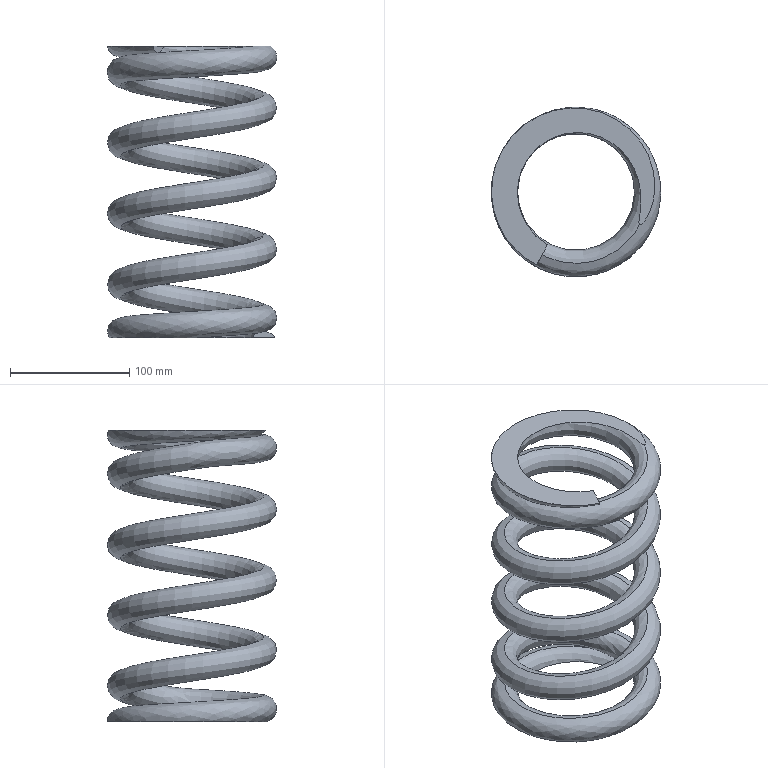Part | STEP file | Helical spring_22X120X280 stiffness 222 | 1 solid | 6 faces | box 142 x 142 x 244.587 mm | volume 741236 mm3 | plane 4 | spline 2